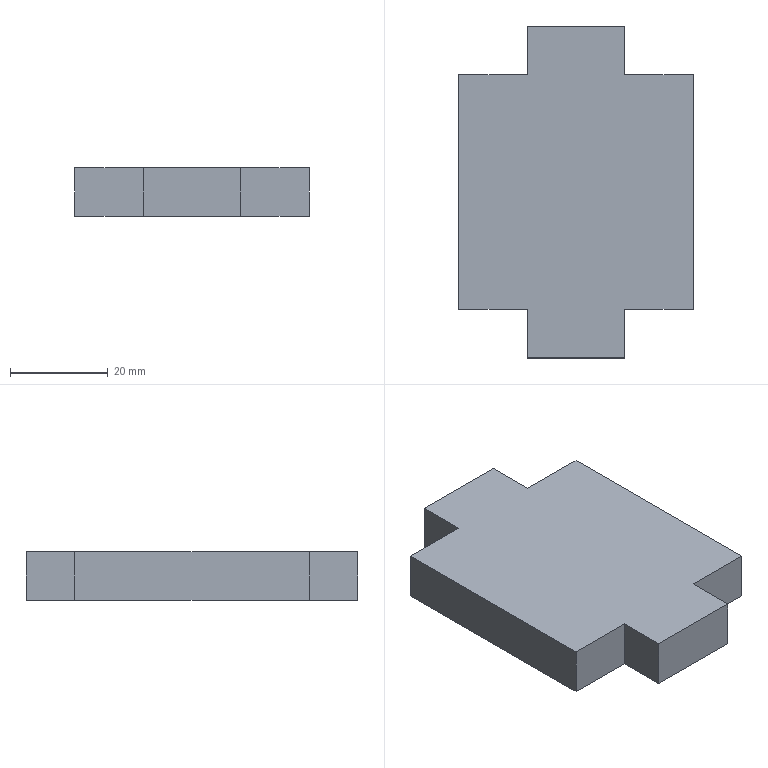Part | SolidWorks | features Extrusion 1, ICE 1 | 1 solid | 14 faces | box 48 x 68 x 10 mm | volume 27040 mm3 | plane 14
STEP:
#1=CARTESIAN_POINT('',(24.,-24.,10.));
#2=VERTEX_POINT('',#1);
#3=CARTESIAN_POINT('',(24.,24.,10.));
#4=VERTEX_POINT('',#3);
#5=CARTESIAN_POINT('',(24.,34.,10.));
#6=DIRECTION('',(0.,1.,0.));
#7=VECTOR('',#6,1000.);
#8=LINE('',#5,#7);
#9=EDGE_CURVE('',#2,#4,#8,.T.);
#10=ORIENTED_EDGE('',*,*,#9,.F.);
#11=CARTESIAN_POINT('',(24.,-24.,0.));
#12=VERTEX_POINT('',#11);
#13=CARTESIAN_POINT('',(24.,-24.,10.));
#14=DIRECTION('',(0.,0.,-1.));
#15=VECTOR('',#14,1000.);
#16=LINE('',#13,#15);
#17=EDGE_CURVE('',#2,#12,#16,.T.);
#18=ORIENTED_EDGE('',*,*,#17,.T.);
#19=CARTESIAN_POINT('',(24.,24.,0.));
#20=VERTEX_POINT('',#19);
#21=CARTESIAN_POINT('',(24.,34.,0.));
#22=DIRECTION('',(0.,1.,0.));
#23=VECTOR('',#22,1000.);
#24=LINE('',#21,#23);
#25=EDGE_CURVE('',#12,#20,#24,.T.);
#26=ORIENTED_EDGE('',*,*,#25,.T.);
#27=CARTESIAN_POINT('',(24.,24.,10.));
#28=DIRECTION('',(0.,0.,1.));
#29=VECTOR('',#28,1000.);
#30=LINE('',#27,#29);
#31=EDGE_CURVE('',#20,#4,#30,.T.);
#32=ORIENTED_EDGE('',*,*,#31,.T.);
#33=EDGE_LOOP('',(#10,#18,#26,#32));
#34=FACE_OUTER_BOUND('',#33,.T.);
#35=CARTESIAN_POINT('',(24.,34.,10.));
#36=DIRECTION('',(-1.,0.,0.));
#37=DIRECTION('',(0.,-1.,0.));
#38=AXIS2_PLACEMENT_3D('',#35,#36,#37);
#39=PLANE('',#38);
#40=ADVANCED_FACE('',(#34),#39,.F.);
#41=CARTESIAN_POINT('',(10.,34.,10.));
#42=VERTEX_POINT('',#41);
#43=CARTESIAN_POINT('',(-10.,34.,10.));
#44=VERTEX_POINT('',#43);
#45=CARTESIAN_POINT('',(-24.,34.,10.));
#46=DIRECTION('',(-1.,0.,0.));
#47=VECTOR('',#46,1000.);
#48=LINE('',#45,#47);
#49=EDGE_CURVE('',#42,#44,#48,.T.);
#50=ORIENTED_EDGE('',*,*,#49,.F.);
#51=CARTESIAN_POINT('',(10.,34.,0.));
#52=VERTEX_POINT('',#51);
#53=CARTESIAN_POINT('',(10.,34.,10.));
#54=DIRECTION('',(0.,0.,-1.));
#55=VECTOR('',#54,1000.);
#56=LINE('',#53,#55);
#57=EDGE_CURVE('',#42,#52,#56,.T.);
#58=ORIENTED_EDGE('',*,*,#57,.T.);
#59=CARTESIAN_POINT('',(-10.,34.,0.));
#60=VERTEX_POINT('',#59);
#61=CARTESIAN_POINT('',(-24.,34.,0.));
#62=DIRECTION('',(-1.,0.,0.));
#63=VECTOR('',#62,1000.);
#64=LINE('',#61,#63);
#65=EDGE_CURVE('',#52,#60,#64,.T.);
#66=ORIENTED_EDGE('',*,*,#65,.T.);
#67=CARTESIAN_POINT('',(-10.,34.,10.));
#68=DIRECTION('',(0.,0.,1.));
#69=VECTOR('',#68,1000.);
#70=LINE('',#67,#69);
#71=EDGE_CURVE('',#60,#44,#70,.T.);
#72=ORIENTED_EDGE('',*,*,#71,.T.);
#73=EDGE_LOOP('',(#50,#58,#66,#72));
#74=FACE_OUTER_BOUND('',#73,.T.);
#75=CARTESIAN_POINT('',(-24.,34.,10.));
#76=DIRECTION('',(0.,-1.,0.));
#77=DIRECTION('',(0.,0.,-1.));
#78=AXIS2_PLACEMENT_3D('',#75,#76,#77);
#79=PLANE('',#78);
#80=ADVANCED_FACE('',(#74),#79,.F.);
#81=CARTESIAN_POINT('',(-24.,24.,0.));
#82=VERTEX_POINT('',#81);
#83=CARTESIAN_POINT('',(-24.,-24.,0.));
#84=VERTEX_POINT('',#83);
#85=CARTESIAN_POINT('',(-24.,34.,0.));
#86=DIRECTION('',(0.,-1.,0.));
#87=VECTOR('',#86,1000.);
#88=LINE('',#85,#87);
#89=EDGE_CURVE('',#82,#84,#88,.T.);
#90=ORIENTED_EDGE('',*,*,#89,.T.);
#91=CARTESIAN_POINT('',(-24.,-24.,10.));
#92=VERTEX_POINT('',#91);
#93=CARTESIAN_POINT('',(-24.,-24.,10.));
#94=DIRECTION('',(0.,0.,1.));
#95=VECTOR('',#94,1000.);
#96=LINE('',#93,#95);
#97=EDGE_CURVE('',#84,#92,#96,.T.);
#98=ORIENTED_EDGE('',*,*,#97,.T.);
#99=CARTESIAN_POINT('',(-24.,24.,10.));
#100=VERTEX_POINT('',#99);
#101=CARTESIAN_POINT('',(-24.,34.,10.));
#102=DIRECTION('',(0.,-1.,0.));
#103=VECTOR('',#102,1000.);
#104=LINE('',#101,#103);
#105=EDGE_CURVE('',#100,#92,#104,.T.);
#106=ORIENTED_EDGE('',*,*,#105,.F.);
#107=CARTESIAN_POINT('',(-24.,24.,10.));
#108=DIRECTION('',(0.,0.,-1.));
#109=VECTOR('',#108,1000.);
#110=LINE('',#107,#109);
#111=EDGE_CURVE('',#100,#82,#110,.T.);
#112=ORIENTED_EDGE('',*,*,#111,.T.);
#113=EDGE_LOOP('',(#90,#98,#106,#112));
#114=FACE_OUTER_BOUND('',#113,.T.);
#115=CARTESIAN_POINT('',(-24.,34.,10.));
#116=DIRECTION('',(1.,0.,0.));
#117=DIRECTION('',(0.,1.,0.));
#118=AXIS2_PLACEMENT_3D('',#115,#116,#117);
#119=PLANE('',#118);
#120=ADVANCED_FACE('',(#114),#119,.F.);
#121=CARTESIAN_POINT('',(-10.,-34.,10.));
#122=VERTEX_POINT('',#121);
#123=CARTESIAN_POINT('',(10.,-34.,10.));
#124=VERTEX_POINT('',#123);
#125=CARTESIAN_POINT('',(-24.,-34.,10.));
#126=DIRECTION('',(1.,0.,0.));
#127=VECTOR('',#126,1000.);
#128=LINE('',#125,#127);
#129=EDGE_CURVE('',#122,#124,#128,.T.);
#130=ORIENTED_EDGE('',*,*,#129,.F.);
#131=CARTESIAN_POINT('',(-10.,-34.,0.));
#132=VERTEX_POINT('',#131);
#133=CARTESIAN_POINT('',(-10.,-34.,10.));
#134=DIRECTION('',(0.,0.,-1.));
#135=VECTOR('',#134,1000.);
#136=LINE('',#133,#135);
#137=EDGE_CURVE('',#122,#132,#136,.T.);
#138=ORIENTED_EDGE('',*,*,#137,.T.);
#139=CARTESIAN_POINT('',(10.,-34.,0.));
#140=VERTEX_POINT('',#139);
#141=CARTESIAN_POINT('',(-24.,-34.,0.));
#142=DIRECTION('',(1.,0.,0.));
#143=VECTOR('',#142,1000.);
#144=LINE('',#141,#143);
#145=EDGE_CURVE('',#132,#140,#144,.T.);
#146=ORIENTED_EDGE('',*,*,#145,.T.);
#147=CARTESIAN_POINT('',(10.,-34.,10.));
#148=DIRECTION('',(0.,0.,1.));
#149=VECTOR('',#148,1000.);
#150=LINE('',#147,#149);
#151=EDGE_CURVE('',#140,#124,#150,.T.);
#152=ORIENTED_EDGE('',*,*,#151,.T.);
#153=EDGE_LOOP('',(#130,#138,#146,#152));
#154=FACE_OUTER_BOUND('',#153,.T.);
#155=CARTESIAN_POINT('',(-24.,-34.,10.));
#156=DIRECTION('',(0.,1.,0.));
#157=DIRECTION('',(0.,0.,1.));
#158=AXIS2_PLACEMENT_3D('',#155,#156,#157);
#159=PLANE('',#158);
#160=ADVANCED_FACE('',(#154),#159,.F.);
#161=CARTESIAN_POINT('',(-10.,-24.,10.));
#162=VERTEX_POINT('',#161);
#163=CARTESIAN_POINT('',(-38.,-24.,10.));
#164=DIRECTION('',(-1.,0.,0.));
#165=VECTOR('',#164,1000.);
#166=LINE('',#163,#165);
#167=EDGE_CURVE('',#162,#92,#166,.T.);
#168=ORIENTED_EDGE('',*,*,#167,.F.);
#169=CARTESIAN_POINT('',(-10.,-44.,10.));
#170=DIRECTION('',(0.,1.,0.));
#171=VECTOR('',#170,1000.);
#172=LINE('',#169,#171);
#173=EDGE_CURVE('',#122,#162,#172,.T.);
#174=ORIENTED_EDGE('',*,*,#173,.F.);
#175=ORIENTED_EDGE('',*,*,#129,.T.);
#176=CARTESIAN_POINT('',(10.,-24.,10.));
#177=VERTEX_POINT('',#176);
#178=CARTESIAN_POINT('',(10.,-44.,10.));
#179=DIRECTION('',(0.,-1.,0.));
#180=VECTOR('',#179,1000.);
#181=LINE('',#178,#180);
#182=EDGE_CURVE('',#177,#124,#181,.T.);
#183=ORIENTED_EDGE('',*,*,#182,.F.);
#184=CARTESIAN_POINT('',(38.,-24.,10.));
#185=DIRECTION('',(-1.,0.,0.));
#186=VECTOR('',#185,1000.);
#187=LINE('',#184,#186);
#188=EDGE_CURVE('',#2,#177,#187,.T.);
#189=ORIENTED_EDGE('',*,*,#188,.F.);
#190=ORIENTED_EDGE('',*,*,#9,.T.);
#191=CARTESIAN_POINT('',(10.,24.,10.));
#192=VERTEX_POINT('',#191);
#193=CARTESIAN_POINT('',(38.,24.,10.));
#194=DIRECTION('',(1.,0.,0.));
#195=VECTOR('',#194,1000.);
#196=LINE('',#193,#195);
#197=EDGE_CURVE('',#192,#4,#196,.T.);
#198=ORIENTED_EDGE('',*,*,#197,.F.);
#199=CARTESIAN_POINT('',(10.,44.,10.));
#200=DIRECTION('',(0.,-1.,0.));
#201=VECTOR('',#200,1000.);
#202=LINE('',#199,#201);
#203=EDGE_CURVE('',#42,#192,#202,.T.);
#204=ORIENTED_EDGE('',*,*,#203,.F.);
#205=ORIENTED_EDGE('',*,*,#49,.T.);
#206=CARTESIAN_POINT('',(-10.,24.,10.));
#207=VERTEX_POINT('',#206);
#208=CARTESIAN_POINT('',(-10.,44.,10.));
#209=DIRECTION('',(0.,1.,0.));
#210=VECTOR('',#209,1000.);
#211=LINE('',#208,#210);
#212=EDGE_CURVE('',#207,#44,#211,.T.);
#213=ORIENTED_EDGE('',*,*,#212,.F.);
#214=CARTESIAN_POINT('',(-38.,24.,10.));
#215=DIRECTION('',(1.,0.,0.));
#216=VECTOR('',#215,1000.);
#217=LINE('',#214,#216);
#218=EDGE_CURVE('',#100,#207,#217,.T.);
#219=ORIENTED_EDGE('',*,*,#218,.F.);
#220=ORIENTED_EDGE('',*,*,#105,.T.);
#221=EDGE_LOOP('',(#168,#174,#175,#183,#189,#190,#198,#204,#205,#213,#219,#220));
#222=FACE_OUTER_BOUND('',#221,.T.);
#223=CARTESIAN_POINT('',(0.,0.,10.));
#224=DIRECTION('',(0.,0.,1.));
#225=DIRECTION('',(1.,0.,0.));
#226=AXIS2_PLACEMENT_3D('',#223,#224,#225);
#227=PLANE('',#226);
#228=ADVANCED_FACE('',(#222),#227,.T.);
#229=CARTESIAN_POINT('',(-10.,-24.,0.));
#230=VERTEX_POINT('',#229);
#231=CARTESIAN_POINT('',(-10.,0.,0.));
#232=DIRECTION('',(0.,1.,0.));
#233=VECTOR('',#232,1000.);
#234=LINE('',#231,#233);
#235=EDGE_CURVE('',#132,#230,#234,.T.);
#236=ORIENTED_EDGE('',*,*,#235,.T.);
#237=CARTESIAN_POINT('',(-38.,-24.,0.));
#238=DIRECTION('',(-1.,0.,0.));
#239=VECTOR('',#238,1000.);
#240=LINE('',#237,#239);
#241=EDGE_CURVE('',#230,#84,#240,.T.);
#242=ORIENTED_EDGE('',*,*,#241,.T.);
#243=ORIENTED_EDGE('',*,*,#89,.F.);
#244=CARTESIAN_POINT('',(-10.,24.,0.));
#245=VERTEX_POINT('',#244);
#246=CARTESIAN_POINT('',(0.,24.,0.));
#247=DIRECTION('',(1.,0.,0.));
#248=VECTOR('',#247,1000.);
#249=LINE('',#246,#248);
#250=EDGE_CURVE('',#82,#245,#249,.T.);
#251=ORIENTED_EDGE('',*,*,#250,.T.);
#252=CARTESIAN_POINT('',(-10.,44.,0.));
#253=DIRECTION('',(0.,1.,0.));
#254=VECTOR('',#253,1000.);
#255=LINE('',#252,#254);
#256=EDGE_CURVE('',#245,#60,#255,.T.);
#257=ORIENTED_EDGE('',*,*,#256,.T.);
#258=ORIENTED_EDGE('',*,*,#65,.F.);
#259=CARTESIAN_POINT('',(10.,24.,0.));
#260=VERTEX_POINT('',#259);
#261=CARTESIAN_POINT('',(10.,0.,0.));
#262=DIRECTION('',(0.,-1.,0.));
#263=VECTOR('',#262,1000.);
#264=LINE('',#261,#263);
#265=EDGE_CURVE('',#52,#260,#264,.T.);
#266=ORIENTED_EDGE('',*,*,#265,.T.);
#267=CARTESIAN_POINT('',(38.,24.,0.));
#268=DIRECTION('',(1.,0.,0.));
#269=VECTOR('',#268,1000.);
#270=LINE('',#267,#269);
#271=EDGE_CURVE('',#260,#20,#270,.T.);
#272=ORIENTED_EDGE('',*,*,#271,.T.);
#273=ORIENTED_EDGE('',*,*,#25,.F.);
#274=CARTESIAN_POINT('',(10.,-24.,0.));
#275=VERTEX_POINT('',#274);
#276=CARTESIAN_POINT('',(0.,-24.,0.));
#277=DIRECTION('',(-1.,0.,0.));
#278=VECTOR('',#277,1000.);
#279=LINE('',#276,#278);
#280=EDGE_CURVE('',#12,#275,#279,.T.);
#281=ORIENTED_EDGE('',*,*,#280,.T.);
#282=CARTESIAN_POINT('',(10.,-44.,0.));
#283=DIRECTION('',(0.,-1.,0.));
#284=VECTOR('',#283,1000.);
#285=LINE('',#282,#284);
#286=EDGE_CURVE('',#275,#140,#285,.T.);
#287=ORIENTED_EDGE('',*,*,#286,.T.);
#288=ORIENTED_EDGE('',*,*,#145,.F.);
#289=EDGE_LOOP('',(#236,#242,#243,#251,#257,#258,#266,#272,#273,#281,#287,#288));
#290=FACE_OUTER_BOUND('',#289,.T.);
#291=CARTESIAN_POINT('',(0.,0.,0.));
#292=DIRECTION('',(0.,0.,1.));
#293=DIRECTION('',(1.,0.,0.));
#294=AXIS2_PLACEMENT_3D('',#291,#292,#293);
#295=PLANE('',#294);
#296=ADVANCED_FACE('',(#290),#295,.F.);
#297=ORIENTED_EDGE('',*,*,#256,.F.);
#298=CARTESIAN_POINT('',(-10.,24.,0.));
#299=DIRECTION('',(0.,0.,1.));
#300=VECTOR('',#299,1000.);
#301=LINE('',#298,#300);
#302=EDGE_CURVE('',#245,#207,#301,.T.);
#303=ORIENTED_EDGE('',*,*,#302,.T.);
#304=ORIENTED_EDGE('',*,*,#212,.T.);
#305=ORIENTED_EDGE('',*,*,#71,.F.);
#306=EDGE_LOOP('',(#297,#303,#304,#305));
#307=FACE_OUTER_BOUND('',#306,.T.);
#308=CARTESIAN_POINT('',(-10.,44.,0.));
#309=DIRECTION('',(1.,0.,0.));
#310=DIRECTION('',(0.,1.,0.));
#311=AXIS2_PLACEMENT_3D('',#308,#309,#310);
#312=PLANE('',#311);
#313=ADVANCED_FACE('',(#307),#312,.F.);
#314=ORIENTED_EDGE('',*,*,#218,.T.);
#315=ORIENTED_EDGE('',*,*,#302,.F.);
#316=ORIENTED_EDGE('',*,*,#250,.F.);
#317=ORIENTED_EDGE('',*,*,#111,.F.);
#318=EDGE_LOOP('',(#314,#315,#316,#317));
#319=FACE_OUTER_BOUND('',#318,.T.);
#320=CARTESIAN_POINT('',(-38.,24.,0.));
#321=DIRECTION('',(0.,-1.,0.));
#322=DIRECTION('',(0.,0.,-1.));
#323=AXIS2_PLACEMENT_3D('',#320,#321,#322);
#324=PLANE('',#323);
#325=ADVANCED_FACE('',(#319),#324,.F.);
#326=ORIENTED_EDGE('',*,*,#271,.F.);
#327=CARTESIAN_POINT('',(10.,24.,0.));
#328=DIRECTION('',(0.,0.,1.));
#329=VECTOR('',#328,1000.);
#330=LINE('',#327,#329);
#331=EDGE_CURVE('',#260,#192,#330,.T.);
#332=ORIENTED_EDGE('',*,*,#331,.T.);
#333=ORIENTED_EDGE('',*,*,#197,.T.);
#334=ORIENTED_EDGE('',*,*,#31,.F.);
#335=EDGE_LOOP('',(#326,#332,#333,#334));
#336=FACE_OUTER_BOUND('',#335,.T.);
#337=CARTESIAN_POINT('',(38.,24.,0.));
#338=DIRECTION('',(0.,-1.,0.));
#339=DIRECTION('',(1.,0.,0.));
#340=AXIS2_PLACEMENT_3D('',#337,#338,#339);
#341=PLANE('',#340);
#342=ADVANCED_FACE('',(#336),#341,.F.);
#343=ORIENTED_EDGE('',*,*,#203,.T.);
#344=ORIENTED_EDGE('',*,*,#331,.F.);
#345=ORIENTED_EDGE('',*,*,#265,.F.);
#346=ORIENTED_EDGE('',*,*,#57,.F.);
#347=EDGE_LOOP('',(#343,#344,#345,#346));
#348=FACE_OUTER_BOUND('',#347,.T.);
#349=CARTESIAN_POINT('',(10.,44.,0.));
#350=DIRECTION('',(-1.,0.,0.));
#351=DIRECTION('',(0.,0.,1.));
#352=AXIS2_PLACEMENT_3D('',#349,#350,#351);
#353=PLANE('',#352);
#354=ADVANCED_FACE('',(#348),#353,.F.);
#355=ORIENTED_EDGE('',*,*,#286,.F.);
#356=CARTESIAN_POINT('',(10.,-24.,0.));
#357=DIRECTION('',(0.,0.,1.));
#358=VECTOR('',#357,1000.);
#359=LINE('',#356,#358);
#360=EDGE_CURVE('',#275,#177,#359,.T.);
#361=ORIENTED_EDGE('',*,*,#360,.T.);
#362=ORIENTED_EDGE('',*,*,#182,.T.);
#363=ORIENTED_EDGE('',*,*,#151,.F.);
#364=EDGE_LOOP('',(#355,#361,#362,#363));
#365=FACE_OUTER_BOUND('',#364,.T.);
#366=CARTESIAN_POINT('',(10.,-44.,0.));
#367=DIRECTION('',(-1.,0.,0.));
#368=DIRECTION('',(0.,-1.,0.));
#369=AXIS2_PLACEMENT_3D('',#366,#367,#368);
#370=PLANE('',#369);
#371=ADVANCED_FACE('',(#365),#370,.F.);
#372=ORIENTED_EDGE('',*,*,#188,.T.);
#373=ORIENTED_EDGE('',*,*,#360,.F.);
#374=ORIENTED_EDGE('',*,*,#280,.F.);
#375=ORIENTED_EDGE('',*,*,#17,.F.);
#376=EDGE_LOOP('',(#372,#373,#374,#375));
#377=FACE_OUTER_BOUND('',#376,.T.);
#378=CARTESIAN_POINT('',(38.,-24.,0.));
#379=DIRECTION('',(0.,1.,0.));
#380=DIRECTION('',(-1.,0.,0.));
#381=AXIS2_PLACEMENT_3D('',#378,#379,#380);
#382=PLANE('',#381);
#383=ADVANCED_FACE('',(#377),#382,.F.);
#384=ORIENTED_EDGE('',*,*,#241,.F.);
#385=CARTESIAN_POINT('',(-10.,-24.,0.));
#386=DIRECTION('',(0.,0.,1.));
#387=VECTOR('',#386,1000.);
#388=LINE('',#385,#387);
#389=EDGE_CURVE('',#230,#162,#388,.T.);
#390=ORIENTED_EDGE('',*,*,#389,.T.);
#391=ORIENTED_EDGE('',*,*,#167,.T.);
#392=ORIENTED_EDGE('',*,*,#97,.F.);
#393=EDGE_LOOP('',(#384,#390,#391,#392));
#394=FACE_OUTER_BOUND('',#393,.T.);
#395=CARTESIAN_POINT('',(-38.,-24.,0.));
#396=DIRECTION('',(0.,1.,0.));
#397=DIRECTION('',(0.,0.,1.));
#398=AXIS2_PLACEMENT_3D('',#395,#396,#397);
#399=PLANE('',#398);
#400=ADVANCED_FACE('',(#394),#399,.F.);
#401=ORIENTED_EDGE('',*,*,#173,.T.);
#402=ORIENTED_EDGE('',*,*,#389,.F.);
#403=ORIENTED_EDGE('',*,*,#235,.F.);
#404=ORIENTED_EDGE('',*,*,#137,.F.);
#405=EDGE_LOOP('',(#401,#402,#403,#404));
#406=FACE_OUTER_BOUND('',#405,.T.);
#407=CARTESIAN_POINT('',(-10.,-44.,0.));
#408=DIRECTION('',(1.,0.,0.));
#409=DIRECTION('',(0.,1.,0.));
#410=AXIS2_PLACEMENT_3D('',#407,#408,#409);
#411=PLANE('',#410);
#412=ADVANCED_FACE('',(#406),#411,.F.);
#413=CLOSED_SHELL('',(#40,#80,#120,#160,#228,#296,#313,#325,#342,#354,#371,#383,#400,#412));
#414=MANIFOLD_SOLID_BREP('',#413);
#415=CARTESIAN_POINT('',(0.,0.,0.));
#416=DIRECTION('',(0.,0.,1.));
#417=DIRECTION('',(1.,0.,0.));
#418=AXIS2_PLACEMENT_3D('',#415,#416,#417);
#419=(LENGTH_UNIT()NAMED_UNIT(*)SI_UNIT(.MILLI.,.METRE.));
#420=UNCERTAINTY_MEASURE_WITH_UNIT(LENGTH_MEASURE(0.00001),#419,'','');
#421=(NAMED_UNIT(*)PLANE_ANGLE_UNIT()SI_UNIT($,.RADIAN.));
#422=(NAMED_UNIT(*)SI_UNIT($,.STERADIAN.)SOLID_ANGLE_UNIT());
#423=(GEOMETRIC_REPRESENTATION_CONTEXT(3)GLOBAL_UNCERTAINTY_ASSIGNED_CONTEXT((#420))GLOBAL_UNIT_ASSIGNED_CONTEXT((#419,#421,#422))REPRESENTATION_CONTEXT('',''));
#424=ADVANCED_BREP_SHAPE_REPRESENTATION('',(#414,#418),#423);